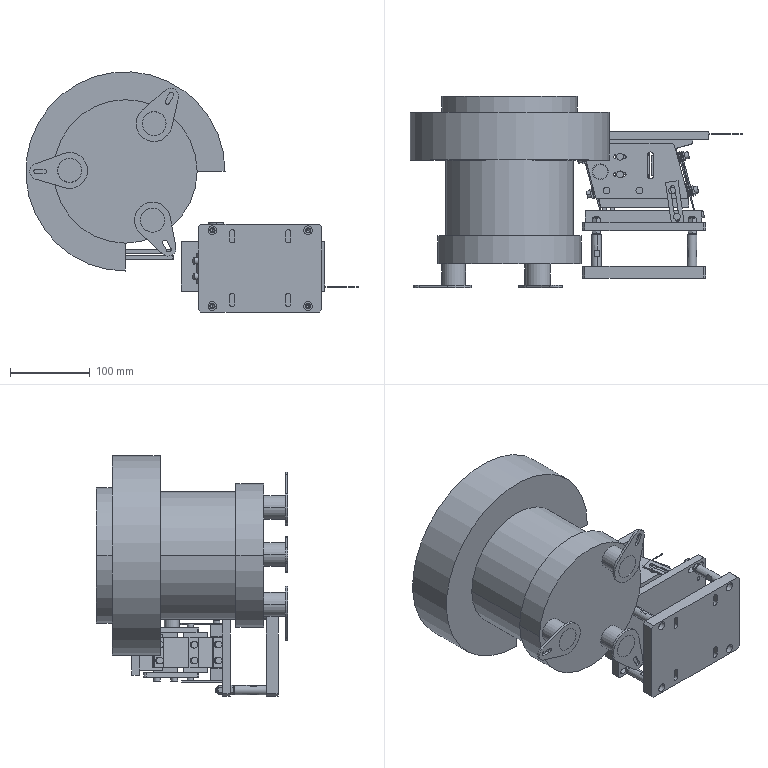Part | SolidWorks | 100 solids | 2026 faces | box 416.776 x 240 x 301.448 mm | volume 7009684 mm3 | plane 1334 | cylinder 537 | cone 155 | commonest cylinder face diameters 6 x121 4.2 x68 5 x68 5.4 x66 8.5 x52 2 x30